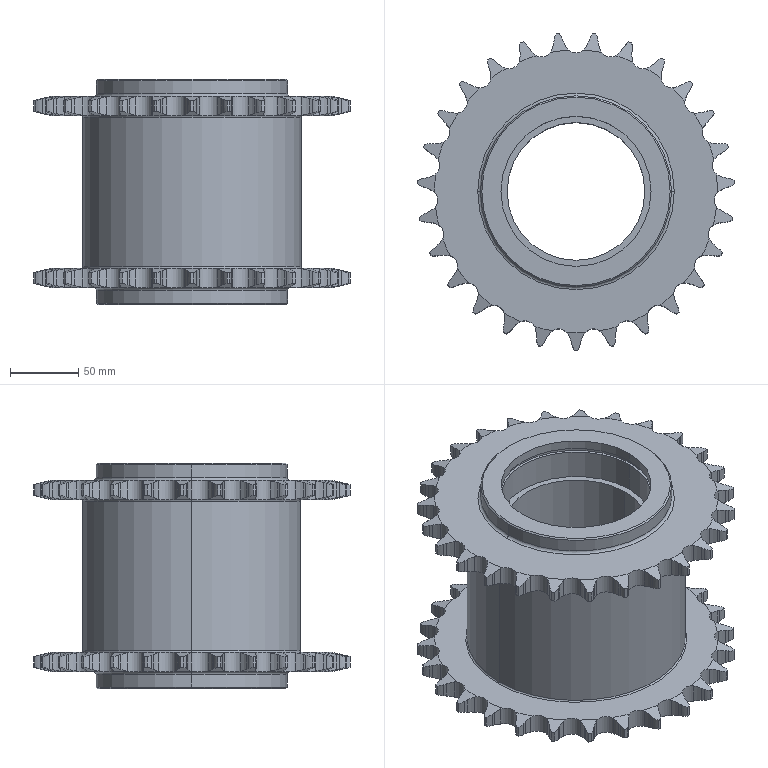Part | STEP file | PCSL50T-5300-03-Driven sprocket 1 | 1 solid | 588 faces | box 232.271 x 231.883 x 165 mm | volume 2210784 mm3 | cylinder 344 | plane 120 | cone 116 | torus 8 | commonest cylinder face diameters 26.077 x108 41.357 x108 15.957 x54 232.551 x54 110 x8 114 x4